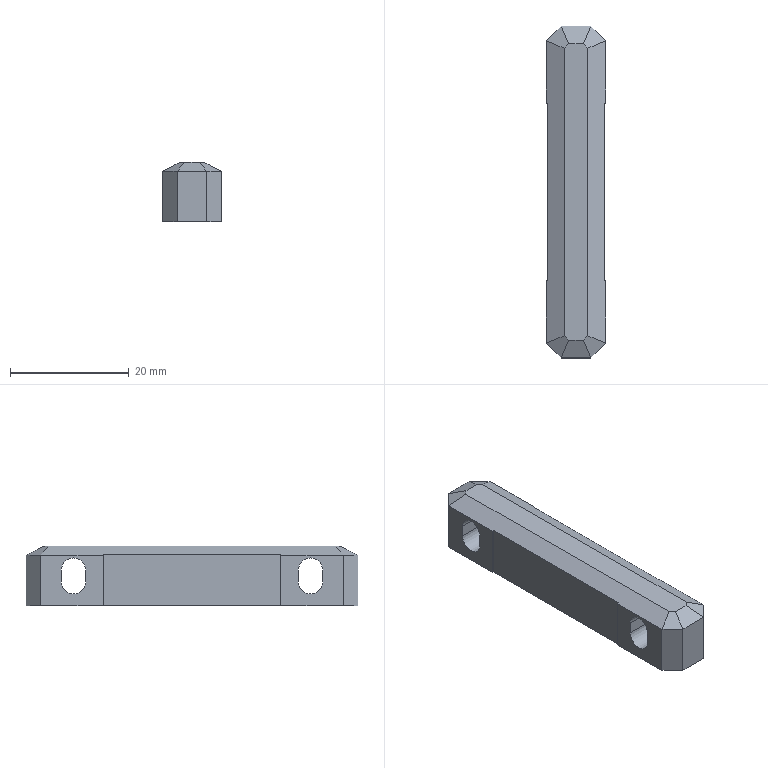Part | STEP file | 2091 Clamp block | 1 solid | 39 faces | box 10 x 56 x 10 mm | volume 4506 mm3 | plane 31 | cylinder 8 | commonest cylinder face diameters 4.1 x6 6 x2